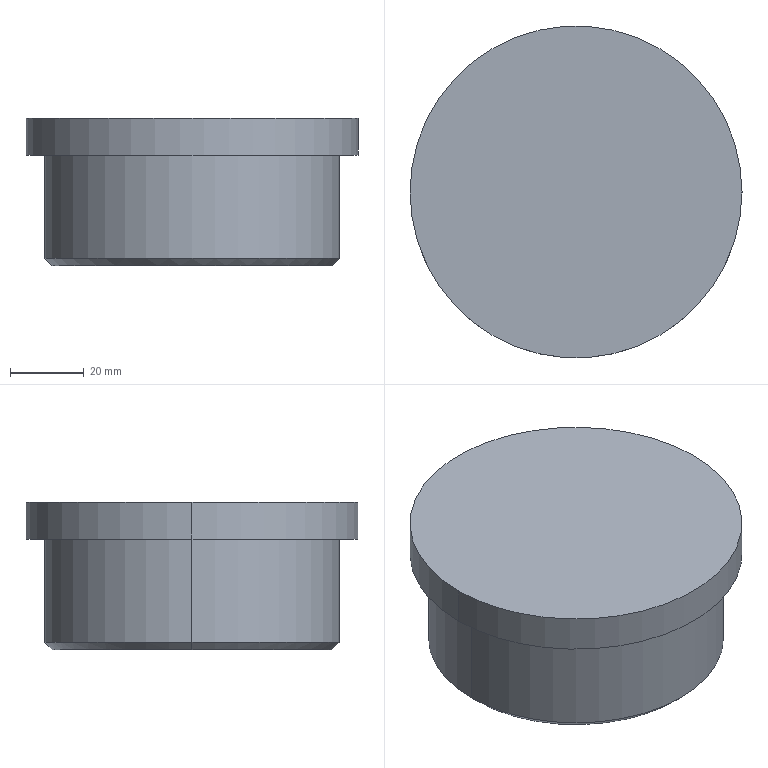Part | SolidWorks | features Chamfer 1, Extrusion 1, ICE 1 | 1 solid | 9 faces | box 90 x 90 x 40 mm | volume 213919 mm3 | cylinder 4 | plane 3 | cone 2 | commonest cylinder face diameters 80 x2 90 x2
STEP:
#1=CARTESIAN_POINT('',(-38.,0.,0.));
#2=VERTEX_POINT('',#1);
#3=CARTESIAN_POINT('',(38.,0.,0.));
#4=VERTEX_POINT('',#3);
#5=CARTESIAN_POINT('',(0.,0.,0.));
#6=DIRECTION('',(0.,0.,-1.));
#7=DIRECTION('',(1.,0.,0.));
#8=AXIS2_PLACEMENT_3D('',#5,#6,#7);
#9=CIRCLE('',#8,38.);
#10=EDGE_CURVE('',#2,#4,#9,.T.);
#11=ORIENTED_EDGE('',*,*,#10,.F.);
#12=CARTESIAN_POINT('',(-40.,0.,2.));
#13=VERTEX_POINT('',#12);
#14=CARTESIAN_POINT('',(-40.,0.,2.));
#15=DIRECTION('',(-0.7071,0.,0.7071));
#16=VECTOR('',#15,1000.);
#17=LINE('',#14,#16);
#18=EDGE_CURVE('',#2,#13,#17,.T.);
#19=ORIENTED_EDGE('',*,*,#18,.T.);
#20=CARTESIAN_POINT('',(40.,0.,2.));
#21=VERTEX_POINT('',#20);
#22=CARTESIAN_POINT('',(0.,0.,2.));
#23=DIRECTION('',(0.,0.,1.));
#24=DIRECTION('',(1.,0.,0.));
#25=AXIS2_PLACEMENT_3D('',#22,#23,#24);
#26=CIRCLE('',#25,40.);
#27=EDGE_CURVE('',#21,#13,#26,.T.);
#28=ORIENTED_EDGE('',*,*,#27,.F.);
#29=CARTESIAN_POINT('',(40.,0.,2.));
#30=DIRECTION('',(0.7071,0.,0.7071));
#31=VECTOR('',#30,1000.);
#32=LINE('',#29,#31);
#33=EDGE_CURVE('',#4,#21,#32,.T.);
#34=ORIENTED_EDGE('',*,*,#33,.F.);
#35=EDGE_LOOP('',(#11,#19,#28,#34));
#36=FACE_OUTER_BOUND('',#35,.T.);
#37=CARTESIAN_POINT('',(0.,0.,2.));
#38=DIRECTION('',(0.,0.,1.));
#39=DIRECTION('',(1.,0.,0.));
#40=AXIS2_PLACEMENT_3D('',#37,#38,#39);
#41=CONICAL_SURFACE('',#40,40.,0.7854);
#42=ADVANCED_FACE('',(#36),#41,.T.);
#43=CARTESIAN_POINT('',(45.,0.,40.));
#44=VERTEX_POINT('',#43);
#45=CARTESIAN_POINT('',(-45.,0.,40.));
#46=VERTEX_POINT('',#45);
#47=CARTESIAN_POINT('',(0.,0.,40.));
#48=DIRECTION('',(0.,0.,1.));
#49=DIRECTION('',(1.,0.,0.));
#50=AXIS2_PLACEMENT_3D('',#47,#48,#49);
#51=CIRCLE('',#50,45.);
#52=EDGE_CURVE('',#44,#46,#51,.T.);
#53=ORIENTED_EDGE('',*,*,#52,.F.);
#54=CARTESIAN_POINT('',(45.,0.,30.));
#55=VERTEX_POINT('',#54);
#56=CARTESIAN_POINT('',(45.,0.,40.));
#57=DIRECTION('',(0.,0.,-1.));
#58=VECTOR('',#57,1000.);
#59=LINE('',#56,#58);
#60=EDGE_CURVE('',#44,#55,#59,.T.);
#61=ORIENTED_EDGE('',*,*,#60,.T.);
#62=CARTESIAN_POINT('',(-45.,0.,30.));
#63=VERTEX_POINT('',#62);
#64=CARTESIAN_POINT('',(0.,0.,30.));
#65=DIRECTION('',(0.,0.,1.));
#66=DIRECTION('',(1.,0.,0.));
#67=AXIS2_PLACEMENT_3D('',#64,#65,#66);
#68=CIRCLE('',#67,45.);
#69=EDGE_CURVE('',#55,#63,#68,.T.);
#70=ORIENTED_EDGE('',*,*,#69,.T.);
#71=CARTESIAN_POINT('',(-45.,0.,40.));
#72=DIRECTION('',(0.,0.,-1.));
#73=VECTOR('',#72,1000.);
#74=LINE('',#71,#73);
#75=EDGE_CURVE('',#46,#63,#74,.T.);
#76=ORIENTED_EDGE('',*,*,#75,.F.);
#77=EDGE_LOOP('',(#53,#61,#70,#76));
#78=FACE_OUTER_BOUND('',#77,.T.);
#79=CARTESIAN_POINT('',(0.,0.,40.));
#80=DIRECTION('',(0.,0.,-1.));
#81=DIRECTION('',(-1.,0.,0.));
#82=AXIS2_PLACEMENT_3D('',#79,#80,#81);
#83=CYLINDRICAL_SURFACE('',#82,45.);
#84=ADVANCED_FACE('',(#78),#83,.T.);
#85=CARTESIAN_POINT('',(40.,0.,30.));
#86=VERTEX_POINT('',#85);
#87=CARTESIAN_POINT('',(-40.,0.,30.));
#88=VERTEX_POINT('',#87);
#89=CARTESIAN_POINT('',(0.,0.,30.));
#90=DIRECTION('',(0.,0.,1.));
#91=DIRECTION('',(1.,0.,0.));
#92=AXIS2_PLACEMENT_3D('',#89,#90,#91);
#93=CIRCLE('',#92,40.);
#94=EDGE_CURVE('',#86,#88,#93,.T.);
#95=ORIENTED_EDGE('',*,*,#94,.F.);
#96=CARTESIAN_POINT('',(40.,0.,30.));
#97=DIRECTION('',(0.,0.,-1.));
#98=VECTOR('',#97,1000.);
#99=LINE('',#96,#98);
#100=EDGE_CURVE('',#86,#21,#99,.T.);
#101=ORIENTED_EDGE('',*,*,#100,.T.);
#102=ORIENTED_EDGE('',*,*,#27,.T.);
#103=CARTESIAN_POINT('',(-40.,0.,30.));
#104=DIRECTION('',(0.,0.,-1.));
#105=VECTOR('',#104,1000.);
#106=LINE('',#103,#105);
#107=EDGE_CURVE('',#88,#13,#106,.T.);
#108=ORIENTED_EDGE('',*,*,#107,.F.);
#109=EDGE_LOOP('',(#95,#101,#102,#108));
#110=FACE_OUTER_BOUND('',#109,.T.);
#111=CARTESIAN_POINT('',(0.,0.,30.));
#112=DIRECTION('',(0.,0.,-1.));
#113=DIRECTION('',(-1.,0.,0.));
#114=AXIS2_PLACEMENT_3D('',#111,#112,#113);
#115=CYLINDRICAL_SURFACE('',#114,40.);
#116=ADVANCED_FACE('',(#110),#115,.T.);
#117=ORIENTED_EDGE('',*,*,#100,.F.);
#118=CARTESIAN_POINT('',(0.,0.,30.));
#119=DIRECTION('',(0.,0.,1.));
#120=DIRECTION('',(1.,0.,0.));
#121=AXIS2_PLACEMENT_3D('',#118,#119,#120);
#122=CIRCLE('',#121,40.);
#123=EDGE_CURVE('',#88,#86,#122,.T.);
#124=ORIENTED_EDGE('',*,*,#123,.F.);
#125=ORIENTED_EDGE('',*,*,#107,.T.);
#126=CARTESIAN_POINT('',(0.,0.,2.));
#127=DIRECTION('',(0.,0.,1.));
#128=DIRECTION('',(1.,0.,0.));
#129=AXIS2_PLACEMENT_3D('',#126,#127,#128);
#130=CIRCLE('',#129,40.);
#131=EDGE_CURVE('',#13,#21,#130,.T.);
#132=ORIENTED_EDGE('',*,*,#131,.T.);
#133=EDGE_LOOP('',(#117,#124,#125,#132));
#134=FACE_OUTER_BOUND('',#133,.T.);
#135=CARTESIAN_POINT('',(0.,0.,30.));
#136=DIRECTION('',(0.,0.,-1.));
#137=DIRECTION('',(-1.,0.,0.));
#138=AXIS2_PLACEMENT_3D('',#135,#136,#137);
#139=CYLINDRICAL_SURFACE('',#138,40.);
#140=ADVANCED_FACE('',(#134),#139,.T.);
#141=CARTESIAN_POINT('',(0.,0.,0.));
#142=DIRECTION('',(0.,0.,-1.));
#143=DIRECTION('',(1.,0.,0.));
#144=AXIS2_PLACEMENT_3D('',#141,#142,#143);
#145=CIRCLE('',#144,38.);
#146=EDGE_CURVE('',#4,#2,#145,.T.);
#147=ORIENTED_EDGE('',*,*,#146,.T.);
#148=ORIENTED_EDGE('',*,*,#10,.T.);
#149=EDGE_LOOP('',(#147,#148));
#150=FACE_OUTER_BOUND('',#149,.T.);
#151=CARTESIAN_POINT('',(0.,0.,0.));
#152=DIRECTION('',(0.,0.,1.));
#153=DIRECTION('',(1.,0.,0.));
#154=AXIS2_PLACEMENT_3D('',#151,#152,#153);
#155=PLANE('',#154);
#156=ADVANCED_FACE('',(#150),#155,.F.);
#157=ORIENTED_EDGE('',*,*,#60,.F.);
#158=CARTESIAN_POINT('',(0.,0.,40.));
#159=DIRECTION('',(0.,0.,1.));
#160=DIRECTION('',(1.,0.,0.));
#161=AXIS2_PLACEMENT_3D('',#158,#159,#160);
#162=CIRCLE('',#161,45.);
#163=EDGE_CURVE('',#46,#44,#162,.T.);
#164=ORIENTED_EDGE('',*,*,#163,.F.);
#165=ORIENTED_EDGE('',*,*,#75,.T.);
#166=CARTESIAN_POINT('',(0.,0.,30.));
#167=DIRECTION('',(0.,0.,1.));
#168=DIRECTION('',(1.,0.,0.));
#169=AXIS2_PLACEMENT_3D('',#166,#167,#168);
#170=CIRCLE('',#169,45.);
#171=EDGE_CURVE('',#63,#55,#170,.T.);
#172=ORIENTED_EDGE('',*,*,#171,.T.);
#173=EDGE_LOOP('',(#157,#164,#165,#172));
#174=FACE_OUTER_BOUND('',#173,.T.);
#175=CARTESIAN_POINT('',(0.,0.,40.));
#176=DIRECTION('',(0.,0.,-1.));
#177=DIRECTION('',(-1.,0.,0.));
#178=AXIS2_PLACEMENT_3D('',#175,#176,#177);
#179=CYLINDRICAL_SURFACE('',#178,45.);
#180=ADVANCED_FACE('',(#174),#179,.T.);
#181=ORIENTED_EDGE('',*,*,#163,.T.);
#182=ORIENTED_EDGE('',*,*,#52,.T.);
#183=EDGE_LOOP('',(#181,#182));
#184=FACE_OUTER_BOUND('',#183,.T.);
#185=CARTESIAN_POINT('',(0.,0.,40.));
#186=DIRECTION('',(0.,0.,1.));
#187=DIRECTION('',(1.,0.,0.));
#188=AXIS2_PLACEMENT_3D('',#185,#186,#187);
#189=PLANE('',#188);
#190=ADVANCED_FACE('',(#184),#189,.T.);
#191=ORIENTED_EDGE('',*,*,#123,.T.);
#192=ORIENTED_EDGE('',*,*,#94,.T.);
#193=EDGE_LOOP('',(#191,#192));
#194=FACE_BOUND('',#193,.T.);
#195=ORIENTED_EDGE('',*,*,#171,.F.);
#196=ORIENTED_EDGE('',*,*,#69,.F.);
#197=EDGE_LOOP('',(#195,#196));
#198=FACE_OUTER_BOUND('',#197,.T.);
#199=CARTESIAN_POINT('',(0.,0.,30.));
#200=DIRECTION('',(0.,0.,1.));
#201=DIRECTION('',(1.,0.,0.));
#202=AXIS2_PLACEMENT_3D('',#199,#200,#201);
#203=PLANE('',#202);
#204=ADVANCED_FACE('',(#194,#198),#203,.F.);
#205=ORIENTED_EDGE('',*,*,#18,.F.);
#206=ORIENTED_EDGE('',*,*,#146,.F.);
#207=ORIENTED_EDGE('',*,*,#33,.T.);
#208=ORIENTED_EDGE('',*,*,#131,.F.);
#209=EDGE_LOOP('',(#205,#206,#207,#208));
#210=FACE_OUTER_BOUND('',#209,.T.);
#211=CARTESIAN_POINT('',(0.,0.,2.));
#212=DIRECTION('',(0.,0.,1.));
#213=DIRECTION('',(1.,0.,0.));
#214=AXIS2_PLACEMENT_3D('',#211,#212,#213);
#215=CONICAL_SURFACE('',#214,40.,0.7854);
#216=ADVANCED_FACE('',(#210),#215,.T.);
#217=CLOSED_SHELL('',(#42,#84,#116,#140,#156,#180,#190,#204,#216));
#218=MANIFOLD_SOLID_BREP('',#217);
#219=CARTESIAN_POINT('',(0.,0.,0.));
#220=DIRECTION('',(0.,0.,1.));
#221=DIRECTION('',(1.,0.,0.));
#222=AXIS2_PLACEMENT_3D('',#219,#220,#221);
#223=(LENGTH_UNIT()NAMED_UNIT(*)SI_UNIT(.MILLI.,.METRE.));
#224=UNCERTAINTY_MEASURE_WITH_UNIT(LENGTH_MEASURE(0.00001),#223,'','');
#225=(NAMED_UNIT(*)PLANE_ANGLE_UNIT()SI_UNIT($,.RADIAN.));
#226=(NAMED_UNIT(*)SI_UNIT($,.STERADIAN.)SOLID_ANGLE_UNIT());
#227=(GEOMETRIC_REPRESENTATION_CONTEXT(3)GLOBAL_UNCERTAINTY_ASSIGNED_CONTEXT((#224))GLOBAL_UNIT_ASSIGNED_CONTEXT((#223,#225,#226))REPRESENTATION_CONTEXT('',''));
#228=ADVANCED_BREP_SHAPE_REPRESENTATION('',(#218,#222),#227);